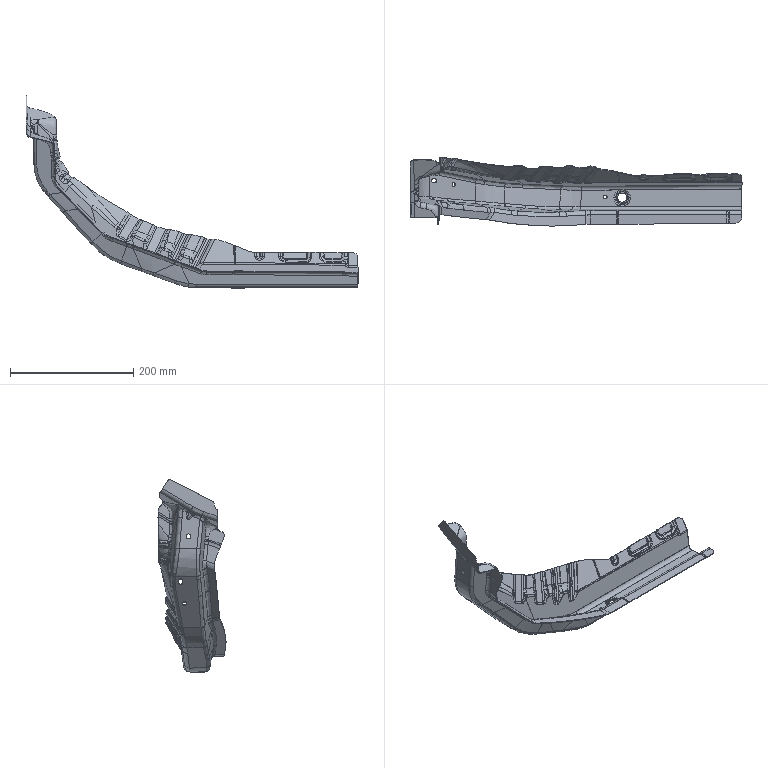Part | 1 solid | 792 faces | box 538.758 x 110.374 x 312.341 mm | volume 123197 mm3 | spline 522 | cylinder 161 | plane 79 | other 16 | sphere 14 | commonest cylinder face diameters 12 x36 14.4 x24 9.6 x12 10 x11 16 x11 13.6 x9